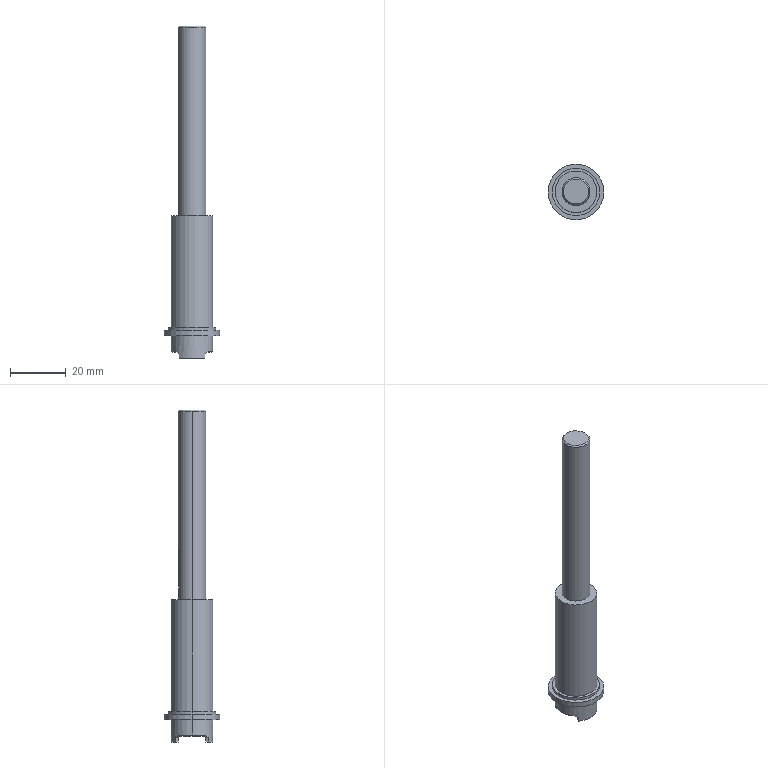Part | STEP file | 11-FG-E03711 | 1 solid | 47 faces | box 20 x 20 x 119 mm | volume 14191 mm3 | plane 19 | cylinder 15 | cone 9 | spline 4 | commonest cylinder face diameters 15 x4 3 x3 3.3 x2 10 x2 17 x2 20 x2
STEP:
#1=CARTESIAN_POINT('',(4.5,0.,119.));
#2=VERTEX_POINT('',#1);
#3=CARTESIAN_POINT('',(-4.5,0.,119.));
#4=VERTEX_POINT('',#3);
#5=CARTESIAN_POINT('',(0.,0.,119.));
#6=DIRECTION('',(0.,0.,1.));
#7=DIRECTION('',(1.,0.,0.));
#8=AXIS2_PLACEMENT_3D('',#5,#6,#7);
#9=CIRCLE('',#8,4.5);
#10=EDGE_CURVE('',#2,#4,#9,.T.);
#11=ORIENTED_EDGE('',*,*,#10,.F.);
#12=CARTESIAN_POINT('',(5.,0.,118.5));
#13=VERTEX_POINT('',#12);
#14=CARTESIAN_POINT('',(4.5,0.,119.));
#15=DIRECTION('',(0.7071,0.,-0.7071));
#16=VECTOR('',#15,1000.);
#17=LINE('',#14,#16);
#18=EDGE_CURVE('',#2,#13,#17,.T.);
#19=ORIENTED_EDGE('',*,*,#18,.T.);
#20=CARTESIAN_POINT('',(-5.,0.,118.5));
#21=VERTEX_POINT('',#20);
#22=CARTESIAN_POINT('',(0.,0.,118.5));
#23=DIRECTION('',(0.,0.,-1.));
#24=DIRECTION('',(1.,0.,0.));
#25=AXIS2_PLACEMENT_3D('',#22,#23,#24);
#26=CIRCLE('',#25,5.);
#27=EDGE_CURVE('',#21,#13,#26,.T.);
#28=ORIENTED_EDGE('',*,*,#27,.F.);
#29=CARTESIAN_POINT('',(-4.5,0.,119.));
#30=DIRECTION('',(-0.7071,0.,-0.7071));
#31=VECTOR('',#30,1000.);
#32=LINE('',#29,#31);
#33=EDGE_CURVE('',#4,#21,#32,.T.);
#34=ORIENTED_EDGE('',*,*,#33,.F.);
#35=EDGE_LOOP('',(#11,#19,#28,#34));
#36=FACE_OUTER_BOUND('',#35,.T.);
#37=CARTESIAN_POINT('',(0.,0.,119.));
#38=DIRECTION('',(0.,0.,-1.));
#39=DIRECTION('',(-1.,0.,0.));
#40=AXIS2_PLACEMENT_3D('',#37,#38,#39);
#41=CONICAL_SURFACE('',#40,4.5,0.7854);
#42=ADVANCED_FACE('',(#36),#41,.T.);
#43=CARTESIAN_POINT('',(1.65,0.,2.5));
#44=VERTEX_POINT('',#43);
#45=CARTESIAN_POINT('',(-1.65,0.,2.5));
#46=VERTEX_POINT('',#45);
#47=CARTESIAN_POINT('',(0.,0.,2.5));
#48=DIRECTION('',(0.,0.,-1.));
#49=DIRECTION('',(-1.,0.,0.));
#50=AXIS2_PLACEMENT_3D('',#47,#48,#49);
#51=CIRCLE('',#50,1.65);
#52=EDGE_CURVE('',#44,#46,#51,.T.);
#53=ORIENTED_EDGE('',*,*,#52,.F.);
#54=CARTESIAN_POINT('',(2.15,0.,2.));
#55=VERTEX_POINT('',#54);
#56=CARTESIAN_POINT('',(1.65,0.,2.5));
#57=DIRECTION('',(0.7071,0.,-0.7071));
#58=VECTOR('',#57,1000.);
#59=LINE('',#56,#58);
#60=EDGE_CURVE('',#44,#55,#59,.T.);
#61=ORIENTED_EDGE('',*,*,#60,.T.);
#62=CARTESIAN_POINT('',(-2.15,0.,2.));
#63=VERTEX_POINT('',#62);
#64=CARTESIAN_POINT('',(0.,0.,2.));
#65=DIRECTION('',(0.,0.,1.));
#66=DIRECTION('',(-1.,0.,0.));
#67=AXIS2_PLACEMENT_3D('',#64,#65,#66);
#68=CIRCLE('',#67,2.15);
#69=EDGE_CURVE('',#63,#55,#68,.T.);
#70=ORIENTED_EDGE('',*,*,#69,.F.);
#71=CARTESIAN_POINT('',(-1.65,0.,2.5));
#72=DIRECTION('',(-0.7071,0.,-0.7071));
#73=VECTOR('',#72,1000.);
#74=LINE('',#71,#73);
#75=EDGE_CURVE('',#46,#63,#74,.T.);
#76=ORIENTED_EDGE('',*,*,#75,.F.);
#77=EDGE_LOOP('',(#53,#61,#70,#76));
#78=FACE_OUTER_BOUND('',#77,.T.);
#79=CARTESIAN_POINT('',(0.,0.,2.5));
#80=DIRECTION('',(0.,0.,-1.));
#81=DIRECTION('',(-1.,0.,0.));
#82=AXIS2_PLACEMENT_3D('',#79,#80,#81);
#83=CONICAL_SURFACE('',#82,1.65,0.7854);
#84=ADVANCED_FACE('',(#78),#83,.F.);
#85=CARTESIAN_POINT('',(7.,0.,2.));
#86=VERTEX_POINT('',#85);
#87=CARTESIAN_POINT('',(5.362,-4.5,2.));
#88=VERTEX_POINT('',#87);
#89=CARTESIAN_POINT('',(0.,0.,2.));
#90=DIRECTION('',(0.,0.,-1.));
#91=DIRECTION('',(-1.,0.,0.));
#92=AXIS2_PLACEMENT_3D('',#89,#90,#91);
#93=CIRCLE('',#92,7.);
#94=EDGE_CURVE('',#86,#88,#93,.T.);
#95=ORIENTED_EDGE('',*,*,#94,.F.);
#96=CARTESIAN_POINT('',(7.5,0.,2.5));
#97=VERTEX_POINT('',#96);
#98=CARTESIAN_POINT('',(7.,0.,2.));
#99=DIRECTION('',(0.7071,0.,0.7071));
#100=VECTOR('',#99,1000.);
#101=LINE('',#98,#100);
#102=EDGE_CURVE('',#86,#97,#101,.T.);
#103=ORIENTED_EDGE('',*,*,#102,.T.);
#104=CARTESIAN_POINT('',(5.745,-4.821,2.5));
#105=VERTEX_POINT('',#104);
#106=CARTESIAN_POINT('',(0.,0.,2.5));
#107=DIRECTION('',(0.,0.,1.));
#108=DIRECTION('',(-1.,0.,0.));
#109=AXIS2_PLACEMENT_3D('',#106,#107,#108);
#110=CIRCLE('',#109,7.5);
#111=EDGE_CURVE('',#105,#97,#110,.T.);
#112=ORIENTED_EDGE('',*,*,#111,.F.);
#113=CARTESIAN_POINT('',(5.362,-4.5,2.));
#114=DIRECTION('',(-0.5416,0.4546,-0.7071));
#115=VECTOR('',#114,1000.);
#116=LINE('',#113,#115);
#117=EDGE_CURVE('',#105,#88,#116,.T.);
#118=ORIENTED_EDGE('',*,*,#117,.T.);
#119=EDGE_LOOP('',(#95,#103,#112,#118));
#120=FACE_OUTER_BOUND('',#119,.T.);
#121=CARTESIAN_POINT('',(0.,0.,2.));
#122=DIRECTION('',(0.,0.,1.));
#123=DIRECTION('',(1.,0.,0.));
#124=AXIS2_PLACEMENT_3D('',#121,#122,#123);
#125=CONICAL_SURFACE('',#124,7.,0.7854);
#126=ADVANCED_FACE('',(#120),#125,.T.);
#127=CARTESIAN_POINT('',(0.,3.,69.5));
#128=VERTEX_POINT('',#127);
#129=CARTESIAN_POINT('',(1.5,3.,68.));
#130=VERTEX_POINT('',#129);
#131=CARTESIAN_POINT('',(0.,3.,68.));
#132=DIRECTION('',(0.,1.,0.));
#133=DIRECTION('',(0.,0.,1.));
#134=AXIS2_PLACEMENT_3D('',#131,#132,#133);
#135=CIRCLE('',#134,1.5);
#136=EDGE_CURVE('',#128,#130,#135,.T.);
#137=ORIENTED_EDGE('',*,*,#136,.F.);
#138=CARTESIAN_POINT('',(0.,5.,69.5));
#139=VERTEX_POINT('',#138);
#140=CARTESIAN_POINT('',(0.,3.,69.5));
#141=DIRECTION('',(0.,1.,0.));
#142=VECTOR('',#141,1000.);
#143=LINE('',#140,#142);
#144=EDGE_CURVE('',#128,#139,#143,.T.);
#145=ORIENTED_EDGE('',*,*,#144,.T.);
#146=CARTESIAN_POINT('',(1.5,4.77,68.));
#147=VERTEX_POINT('',#146);
#148=CARTESIAN_POINT('',(1.5,4.77,68.));
#149=CARTESIAN_POINT('',(1.5,4.77,68.1));
#150=CARTESIAN_POINT('',(1.49,4.773,68.198));
#151=CARTESIAN_POINT('',(1.452,4.785,68.39));
#152=CARTESIAN_POINT('',(1.423,4.794,68.486));
#153=CARTESIAN_POINT('',(1.347,4.815,68.667));
#154=CARTESIAN_POINT('',(1.301,4.828,68.753));
#155=CARTESIAN_POINT('',(1.192,4.856,68.916));
#156=CARTESIAN_POINT('',(1.129,4.871,68.992));
#157=CARTESIAN_POINT('',(0.9226,4.916,69.199));
#158=CARTESIAN_POINT('',(0.7561,4.946,69.31));
#159=CARTESIAN_POINT('',(0.3953,4.988,69.46));
#160=CARTESIAN_POINT('',(0.197,5.,69.5));
#161=CARTESIAN_POINT('',(0.,5.,69.5));
#162=B_SPLINE_CURVE_WITH_KNOTS('',3,(#148,#149,#150,#151,#152,#153,#154,#155,#156,#157,#158,#159,#160,#161),.UNSPECIFIED.,.F.,.F.,(4,2,2,2,2,2,4),(0.,0.0002949,0.0005898,0.0008847,0.00118,0.001769,0.002359),.UNSPECIFIED.);
#163=EDGE_CURVE('',#147,#139,#162,.T.);
#164=ORIENTED_EDGE('',*,*,#163,.F.);
#165=CARTESIAN_POINT('',(1.5,3.,68.));
#166=DIRECTION('',(0.,1.,0.));
#167=VECTOR('',#166,1000.);
#168=LINE('',#165,#167);
#169=EDGE_CURVE('',#130,#147,#168,.T.);
#170=ORIENTED_EDGE('',*,*,#169,.F.);
#171=EDGE_LOOP('',(#137,#145,#164,#170));
#172=FACE_OUTER_BOUND('',#171,.T.);
#173=CARTESIAN_POINT('',(0.,3.,68.));
#174=DIRECTION('',(0.,1.,0.));
#175=DIRECTION('',(0.,0.,1.));
#176=AXIS2_PLACEMENT_3D('',#173,#174,#175);
#177=CYLINDRICAL_SURFACE('',#176,1.5);
#178=ADVANCED_FACE('',(#172),#177,.F.);
#179=CARTESIAN_POINT('',(7.5,0.,51.));
#180=VERTEX_POINT('',#179);
#181=CARTESIAN_POINT('',(-7.5,0.,51.));
#182=VERTEX_POINT('',#181);
#183=CARTESIAN_POINT('',(0.,0.,51.));
#184=DIRECTION('',(0.,0.,1.));
#185=DIRECTION('',(1.,0.,0.));
#186=AXIS2_PLACEMENT_3D('',#183,#184,#185);
#187=CIRCLE('',#186,7.5);
#188=EDGE_CURVE('',#180,#182,#187,.T.);
#189=ORIENTED_EDGE('',*,*,#188,.F.);
#190=CARTESIAN_POINT('',(7.5,0.,11.));
#191=VERTEX_POINT('',#190);
#192=CARTESIAN_POINT('',(7.5,0.,51.));
#193=DIRECTION('',(0.,0.,-1.));
#194=VECTOR('',#193,1000.);
#195=LINE('',#192,#194);
#196=EDGE_CURVE('',#180,#191,#195,.T.);
#197=ORIENTED_EDGE('',*,*,#196,.T.);
#198=CARTESIAN_POINT('',(-7.5,0.,11.));
#199=VERTEX_POINT('',#198);
#200=CARTESIAN_POINT('',(0.,0.,11.));
#201=DIRECTION('',(0.,0.,1.));
#202=DIRECTION('',(1.,0.,0.));
#203=AXIS2_PLACEMENT_3D('',#200,#201,#202);
#204=CIRCLE('',#203,7.5);
#205=EDGE_CURVE('',#191,#199,#204,.T.);
#206=ORIENTED_EDGE('',*,*,#205,.T.);
#207=CARTESIAN_POINT('',(-7.5,0.,51.));
#208=DIRECTION('',(0.,0.,-1.));
#209=VECTOR('',#208,1000.);
#210=LINE('',#207,#209);
#211=EDGE_CURVE('',#182,#199,#210,.T.);
#212=ORIENTED_EDGE('',*,*,#211,.F.);
#213=EDGE_LOOP('',(#189,#197,#206,#212));
#214=FACE_OUTER_BOUND('',#213,.T.);
#215=CARTESIAN_POINT('',(0.,0.,51.));
#216=DIRECTION('',(0.,0.,-1.));
#217=DIRECTION('',(-1.,0.,0.));
#218=AXIS2_PLACEMENT_3D('',#215,#216,#217);
#219=CYLINDRICAL_SURFACE('',#218,7.5);
#220=ADVANCED_FACE('',(#214),#219,.T.);
#221=CARTESIAN_POINT('',(1.5,4.77,53.));
#222=VERTEX_POINT('',#221);
#223=CARTESIAN_POINT('',(1.5,4.77,119.));
#224=DIRECTION('',(0.,0.,1.));
#225=VECTOR('',#224,1000.);
#226=LINE('',#223,#225);
#227=EDGE_CURVE('',#222,#147,#226,.T.);
#228=ORIENTED_EDGE('',*,*,#227,.T.);
#229=ORIENTED_EDGE('',*,*,#163,.T.);
#230=CARTESIAN_POINT('',(-1.5,4.77,68.));
#231=VERTEX_POINT('',#230);
#232=CARTESIAN_POINT('',(0.,5.,69.5));
#233=CARTESIAN_POINT('',(-0.0984,5.,69.5));
#234=CARTESIAN_POINT('',(-0.1984,4.997,69.49));
#235=CARTESIAN_POINT('',(-0.391,4.986,69.451));
#236=CARTESIAN_POINT('',(-0.4848,4.977,69.423));
#237=CARTESIAN_POINT('',(-0.7581,4.946,69.309));
#238=CARTESIAN_POINT('',(-0.9225,4.916,69.199));
#239=CARTESIAN_POINT('',(-1.13,4.871,68.991));
#240=CARTESIAN_POINT('',(-1.192,4.856,68.916));
#241=CARTESIAN_POINT('',(-1.3,4.828,68.754));
#242=CARTESIAN_POINT('',(-1.347,4.815,68.667));
#243=CARTESIAN_POINT('',(-1.46,4.783,68.396));
#244=CARTESIAN_POINT('',(-1.5,4.77,68.199));
#245=CARTESIAN_POINT('',(-1.5,4.77,68.));
#246=B_SPLINE_CURVE_WITH_KNOTS('',3,(#232,#233,#234,#235,#236,#237,#238,#239,#240,#241,#242,#243,#244,#245),.UNSPECIFIED.,.F.,.F.,(4,2,2,2,2,2,4),(0.002359,0.002654,0.002948,0.003537,0.003832,0.004126,0.004715),.UNSPECIFIED.);
#247=EDGE_CURVE('',#139,#231,#246,.T.);
#248=ORIENTED_EDGE('',*,*,#247,.T.);
#249=CARTESIAN_POINT('',(-1.5,4.77,53.));
#250=VERTEX_POINT('',#249);
#251=CARTESIAN_POINT('',(-1.5,4.77,119.));
#252=DIRECTION('',(0.,0.,-1.));
#253=VECTOR('',#252,1000.);
#254=LINE('',#251,#253);
#255=EDGE_CURVE('',#231,#250,#254,.T.);
#256=ORIENTED_EDGE('',*,*,#255,.T.);
#257=CARTESIAN_POINT('',(-1.5,4.77,53.));
#258=CARTESIAN_POINT('',(-1.5,4.77,52.9));
#259=CARTESIAN_POINT('',(-1.49,4.773,52.802));
#260=CARTESIAN_POINT('',(-1.452,4.785,52.61));
#261=CARTESIAN_POINT('',(-1.423,4.794,52.514));
#262=CARTESIAN_POINT('',(-1.347,4.815,52.333));
#263=CARTESIAN_POINT('',(-1.301,4.828,52.247));
#264=CARTESIAN_POINT('',(-1.192,4.856,52.085));
#265=CARTESIAN_POINT('',(-1.129,4.871,52.008));
#266=CARTESIAN_POINT('',(-0.9233,4.916,51.802));
#267=CARTESIAN_POINT('',(-0.7569,4.946,51.69));
#268=CARTESIAN_POINT('',(-0.3965,4.988,51.54));
#269=CARTESIAN_POINT('',(-0.1984,5.,51.5));
#270=CARTESIAN_POINT('',(0.09698,5.,51.5));
#271=CARTESIAN_POINT('',(0.197,4.997,51.51));
#272=CARTESIAN_POINT('',(0.3898,4.986,51.548));
#273=CARTESIAN_POINT('',(0.4837,4.977,51.577));
#274=CARTESIAN_POINT('',(0.7572,4.946,51.69));
#275=CARTESIAN_POINT('',(0.9219,4.916,51.801));
#276=CARTESIAN_POINT('',(1.13,4.871,52.008));
#277=CARTESIAN_POINT('',(1.191,4.856,52.083));
#278=CARTESIAN_POINT('',(1.3,4.828,52.245));
#279=CARTESIAN_POINT('',(1.347,4.815,52.333));
#280=CARTESIAN_POINT('',(1.46,4.783,52.604));
#281=CARTESIAN_POINT('',(1.5,4.77,52.801));
#282=CARTESIAN_POINT('',(1.5,4.77,53.));
#283=B_SPLINE_CURVE_WITH_KNOTS('',3,(#257,#258,#259,#260,#261,#262,#263,#264,#265,#266,#267,#268,#269,#270,#271,#272,#273,#274,#275,#276,#277,#278,#279,#280,#281,#282),.UNSPECIFIED.,.F.,.F.,(4,2,2,2,2,2,2,2,2,2,2,2,4),(0.,0.0002947,0.0005894,0.0008841,0.001179,0.001768,0.002358,0.002652,0.002947,0.003536,0.003831,0.004126,0.004715),.UNSPECIFIED.);
#284=EDGE_CURVE('',#250,#222,#283,.T.);
#285=ORIENTED_EDGE('',*,*,#284,.T.);
#286=EDGE_LOOP('',(#228,#229,#248,#256,#285));
#287=FACE_BOUND('',#286,.T.);
#288=ORIENTED_EDGE('',*,*,#27,.T.);
#289=CARTESIAN_POINT('',(5.,0.,51.));
#290=VERTEX_POINT('',#289);
#291=CARTESIAN_POINT('',(5.,0.,119.));
#292=DIRECTION('',(0.,0.,-1.));
#293=VECTOR('',#292,1000.);
#294=LINE('',#291,#293);
#295=EDGE_CURVE('',#13,#290,#294,.T.);
#296=ORIENTED_EDGE('',*,*,#295,.T.);
#297=CARTESIAN_POINT('',(-5.,0.,51.));
#298=VERTEX_POINT('',#297);
#299=CARTESIAN_POINT('',(0.,0.,51.));
#300=DIRECTION('',(0.,0.,1.));
#301=DIRECTION('',(1.,0.,0.));
#302=AXIS2_PLACEMENT_3D('',#299,#300,#301);
#303=CIRCLE('',#302,5.);
#304=EDGE_CURVE('',#290,#298,#303,.T.);
#305=ORIENTED_EDGE('',*,*,#304,.T.);
#306=CARTESIAN_POINT('',(-5.,0.,119.));
#307=DIRECTION('',(0.,0.,-1.));
#308=VECTOR('',#307,1000.);
#309=LINE('',#306,#308);
#310=EDGE_CURVE('',#21,#298,#309,.T.);
#311=ORIENTED_EDGE('',*,*,#310,.F.);
#312=EDGE_LOOP('',(#288,#296,#305,#311));
#313=FACE_OUTER_BOUND('',#312,.T.);
#314=CARTESIAN_POINT('',(0.,0.,119.));
#315=DIRECTION('',(0.,0.,-1.));
#316=DIRECTION('',(-1.,0.,0.));
#317=AXIS2_PLACEMENT_3D('',#314,#315,#316);
#318=CYLINDRICAL_SURFACE('',#317,5.);
#319=ADVANCED_FACE('',(#287,#313),#318,.T.);
#320=CARTESIAN_POINT('',(8.5,0.,10.));
#321=VERTEX_POINT('',#320);
#322=CARTESIAN_POINT('',(-8.5,0.,10.));
#323=VERTEX_POINT('',#322);
#324=CARTESIAN_POINT('',(0.,0.,10.));
#325=DIRECTION('',(0.,0.,1.));
#326=DIRECTION('',(1.,0.,0.));
#327=AXIS2_PLACEMENT_3D('',#324,#325,#326);
#328=CIRCLE('',#327,8.5);
#329=EDGE_CURVE('',#321,#323,#328,.T.);
#330=ORIENTED_EDGE('',*,*,#329,.T.);
#331=CARTESIAN_POINT('',(-8.5,0.,11.));
#332=VERTEX_POINT('',#331);
#333=CARTESIAN_POINT('',(-8.5,0.,10.));
#334=DIRECTION('',(0.,0.,1.));
#335=VECTOR('',#334,1000.);
#336=LINE('',#333,#335);
#337=EDGE_CURVE('',#323,#332,#336,.T.);
#338=ORIENTED_EDGE('',*,*,#337,.T.);
#339=CARTESIAN_POINT('',(8.5,0.,11.));
#340=VERTEX_POINT('',#339);
#341=CARTESIAN_POINT('',(0.,0.,11.));
#342=DIRECTION('',(0.,0.,1.));
#343=DIRECTION('',(1.,0.,0.));
#344=AXIS2_PLACEMENT_3D('',#341,#342,#343);
#345=CIRCLE('',#344,8.5);
#346=EDGE_CURVE('',#340,#332,#345,.T.);
#347=ORIENTED_EDGE('',*,*,#346,.F.);
#348=CARTESIAN_POINT('',(8.5,0.,10.));
#349=DIRECTION('',(0.,0.,1.));
#350=VECTOR('',#349,1000.);
#351=LINE('',#348,#350);
#352=EDGE_CURVE('',#321,#340,#351,.T.);
#353=ORIENTED_EDGE('',*,*,#352,.F.);
#354=EDGE_LOOP('',(#330,#338,#347,#353));
#355=FACE_OUTER_BOUND('',#354,.T.);
#356=CARTESIAN_POINT('',(0.,0.,10.));
#357=DIRECTION('',(0.,0.,1.));
#358=DIRECTION('',(1.,0.,0.));
#359=AXIS2_PLACEMENT_3D('',#356,#357,#358);
#360=CYLINDRICAL_SURFACE('',#359,8.5);
#361=ADVANCED_FACE('',(#355),#360,.T.);
#362=CARTESIAN_POINT('',(1.65,0.,13.5));
#363=VERTEX_POINT('',#362);
#364=CARTESIAN_POINT('',(-1.65,0.,13.5));
#365=VERTEX_POINT('',#364);
#366=CARTESIAN_POINT('',(0.,0.,13.5));
#367=DIRECTION('',(0.,0.,-1.));
#368=DIRECTION('',(-1.,0.,0.));
#369=AXIS2_PLACEMENT_3D('',#366,#367,#368);
#370=CIRCLE('',#369,1.65);
#371=EDGE_CURVE('',#363,#365,#370,.T.);
#372=ORIENTED_EDGE('',*,*,#371,.F.);
#373=CARTESIAN_POINT('',(1.65,0.,2.));
#374=DIRECTION('',(0.,0.,-1.));
#375=VECTOR('',#374,1000.);
#376=LINE('',#373,#375);
#377=EDGE_CURVE('',#363,#44,#376,.T.);
#378=ORIENTED_EDGE('',*,*,#377,.T.);
#379=ORIENTED_EDGE('',*,*,#52,.T.);
#380=CARTESIAN_POINT('',(-1.65,0.,2.));
#381=DIRECTION('',(0.,0.,-1.));
#382=VECTOR('',#381,1000.);
#383=LINE('',#380,#382);
#384=EDGE_CURVE('',#365,#46,#383,.T.);
#385=ORIENTED_EDGE('',*,*,#384,.F.);
#386=EDGE_LOOP('',(#372,#378,#379,#385));
#387=FACE_OUTER_BOUND('',#386,.T.);
#388=CARTESIAN_POINT('',(0.,0.,2.));
#389=DIRECTION('',(0.,0.,-1.));
#390=DIRECTION('',(-1.,0.,0.));
#391=AXIS2_PLACEMENT_3D('',#388,#389,#390);
#392=CYLINDRICAL_SURFACE('',#391,1.65);
#393=ADVANCED_FACE('',(#387),#392,.F.);
#394=CARTESIAN_POINT('',(0.,0.,14.491));
#395=VERTEX_POINT('',#394);
#396=CARTESIAN_POINT('',(-1.65,0.,13.5));
#397=DIRECTION('',(-0.8572,0.,-0.515));
#398=VECTOR('',#397,1000.);
#399=LINE('',#396,#398);
#400=EDGE_CURVE('',#395,#365,#399,.T.);
#401=ORIENTED_EDGE('',*,*,#400,.F.);
#402=CARTESIAN_POINT('',(1.65,0.,13.5));
#403=DIRECTION('',(0.8572,0.,-0.515));
#404=VECTOR('',#403,1000.);
#405=LINE('',#402,#404);
#406=EDGE_CURVE('',#395,#363,#405,.T.);
#407=ORIENTED_EDGE('',*,*,#406,.T.);
#408=ORIENTED_EDGE('',*,*,#371,.T.);
#409=EDGE_LOOP('',(#401,#407,#408));
#410=FACE_OUTER_BOUND('',#409,.T.);
#411=CARTESIAN_POINT('',(0.,0.,13.5));
#412=DIRECTION('',(0.,0.,-1.));
#413=DIRECTION('',(-1.,0.,0.));
#414=AXIS2_PLACEMENT_3D('',#411,#412,#413);
#415=CONICAL_SURFACE('',#414,1.65,1.03);
#416=ADVANCED_FACE('',(#410),#415,.F.);
#417=CARTESIAN_POINT('',(7.5,0.,8.));
#418=VERTEX_POINT('',#417);
#419=CARTESIAN_POINT('',(-7.5,0.,8.));
#420=VERTEX_POINT('',#419);
#421=CARTESIAN_POINT('',(0.,0.,8.));
#422=DIRECTION('',(0.,0.,1.));
#423=DIRECTION('',(1.,0.,0.));
#424=AXIS2_PLACEMENT_3D('',#421,#422,#423);
#425=CIRCLE('',#424,7.5);
#426=EDGE_CURVE('',#418,#420,#425,.T.);
#427=ORIENTED_EDGE('',*,*,#426,.F.);
#428=CARTESIAN_POINT('',(7.5,0.,8.));
#429=DIRECTION('',(0.,0.,-1.));
#430=VECTOR('',#429,1000.);
#431=LINE('',#428,#430);
#432=EDGE_CURVE('',#418,#97,#431,.T.);
#433=ORIENTED_EDGE('',*,*,#432,.T.);
#434=CARTESIAN_POINT('',(5.745,4.821,2.5));
#435=VERTEX_POINT('',#434);
#436=CARTESIAN_POINT('',(0.,0.,2.5));
#437=DIRECTION('',(0.,0.,1.));
#438=DIRECTION('',(-1.,0.,0.));
#439=AXIS2_PLACEMENT_3D('',#436,#437,#438);
#440=CIRCLE('',#439,7.5);
#441=EDGE_CURVE('',#97,#435,#440,.T.);
#442=ORIENTED_EDGE('',*,*,#441,.T.);
#443=CARTESIAN_POINT('',(4.639,5.893,1.5));
#444=VERTEX_POINT('',#443);
#445=CARTESIAN_POINT('',(4.639,5.893,1.5));
#446=CARTESIAN_POINT('',(4.839,5.736,1.672));
#447=CARTESIAN_POINT('',(5.029,5.57,1.845));
#448=CARTESIAN_POINT('',(5.397,5.215,2.185));
#449=CARTESIAN_POINT('',(5.572,5.027,2.352));
#450=CARTESIAN_POINT('',(5.745,4.821,2.5));
#451=B_SPLINE_CURVE_WITH_KNOTS('',3,(#445,#446,#447,#448,#449,#450),.UNSPECIFIED.,.F.,.F.,(4,2,4),(0.,0.0009195,0.001839),.UNSPECIFIED.);
#452=EDGE_CURVE('',#444,#435,#451,.T.);
#453=ORIENTED_EDGE('',*,*,#452,.F.);
#454=CARTESIAN_POINT('',(4.639,5.893,0.));
#455=VERTEX_POINT('',#454);
#456=CARTESIAN_POINT('',(4.639,5.893,8.));
#457=DIRECTION('',(0.,0.,-1.));
#458=VECTOR('',#457,1000.);
#459=LINE('',#456,#458);
#460=EDGE_CURVE('',#444,#455,#459,.T.);
#461=ORIENTED_EDGE('',*,*,#460,.T.);
#462=CARTESIAN_POINT('',(-4.639,5.893,0.));
#463=VERTEX_POINT('',#462);
#464=CARTESIAN_POINT('',(0.,0.,0.));
#465=DIRECTION('',(0.,0.,1.));
#466=DIRECTION('',(1.,0.,0.));
#467=AXIS2_PLACEMENT_3D('',#464,#465,#466);
#468=CIRCLE('',#467,7.5);
#469=EDGE_CURVE('',#455,#463,#468,.T.);
#470=ORIENTED_EDGE('',*,*,#469,.T.);
#471=CARTESIAN_POINT('',(-4.639,5.893,1.5));
#472=VERTEX_POINT('',#471);
#473=CARTESIAN_POINT('',(-4.639,5.893,8.));
#474=DIRECTION('',(0.,0.,1.));
#475=VECTOR('',#474,1000.);
#476=LINE('',#473,#475);
#477=EDGE_CURVE('',#463,#472,#476,.T.);
#478=ORIENTED_EDGE('',*,*,#477,.T.);
#479=CARTESIAN_POINT('',(-5.745,4.821,2.5));
#480=VERTEX_POINT('',#479);
#481=CARTESIAN_POINT('',(-5.745,4.821,2.5));
#482=CARTESIAN_POINT('',(-5.572,5.027,2.352));
#483=CARTESIAN_POINT('',(-5.396,5.215,2.185));
#484=CARTESIAN_POINT('',(-5.029,5.57,1.845));
#485=CARTESIAN_POINT('',(-4.839,5.736,1.672));
#486=CARTESIAN_POINT('',(-4.639,5.893,1.5));
#487=B_SPLINE_CURVE_WITH_KNOTS('',3,(#481,#482,#483,#484,#485,#486),.UNSPECIFIED.,.F.,.F.,(4,2,4),(0.,0.0009192,0.001838),.UNSPECIFIED.);
#488=EDGE_CURVE('',#480,#472,#487,.T.);
#489=ORIENTED_EDGE('',*,*,#488,.F.);
#490=CARTESIAN_POINT('',(-7.5,0.,2.5));
#491=VERTEX_POINT('',#490);
#492=CARTESIAN_POINT('',(0.,0.,2.5));
#493=DIRECTION('',(0.,0.,1.));
#494=DIRECTION('',(-1.,0.,0.));
#495=AXIS2_PLACEMENT_3D('',#492,#493,#494);
#496=CIRCLE('',#495,7.5);
#497=EDGE_CURVE('',#480,#491,#496,.T.);
#498=ORIENTED_EDGE('',*,*,#497,.T.);
#499=CARTESIAN_POINT('',(-7.5,0.,8.));
#500=DIRECTION('',(0.,0.,-1.));
#501=VECTOR('',#500,1000.);
#502=LINE('',#499,#501);
#503=EDGE_CURVE('',#420,#491,#502,.T.);
#504=ORIENTED_EDGE('',*,*,#503,.F.);
#505=EDGE_LOOP('',(#427,#433,#442,#453,#461,#470,#478,#489,#498,#504));
#506=FACE_OUTER_BOUND('',#505,.T.);
#507=CARTESIAN_POINT('',(0.,0.,8.));
#508=DIRECTION('',(0.,0.,-1.));
#509=DIRECTION('',(-1.,0.,0.));
#510=AXIS2_PLACEMENT_3D('',#507,#508,#509);
#511=CYLINDRICAL_SURFACE('',#510,7.5);
#512=ADVANCED_FACE('',(#506),#511,.T.);
#513=CARTESIAN_POINT('',(10.,0.,10.));
#514=VERTEX_POINT('',#513);
#515=CARTESIAN_POINT('',(-10.,0.,10.));
#516=VERTEX_POINT('',#515);
#517=CARTESIAN_POINT('',(0.,0.,10.));
#518=DIRECTION('',(0.,0.,1.));
#519=DIRECTION('',(1.,0.,0.));
#520=AXIS2_PLACEMENT_3D('',#517,#518,#519);
#521=CIRCLE('',#520,10.);
#522=EDGE_CURVE('',#514,#516,#521,.T.);
#523=ORIENTED_EDGE('',*,*,#522,.F.);
#524=CARTESIAN_POINT('',(10.,0.,8.));
#525=VERTEX_POINT('',#524);
#526=CARTESIAN_POINT('',(10.,0.,11.));
#527=DIRECTION('',(0.,0.,-1.));
#528=VECTOR('',#527,1000.);
#529=LINE('',#526,#528);
#530=EDGE_CURVE('',#514,#525,#529,.T.);
#531=ORIENTED_EDGE('',*,*,#530,.T.);
#532=CARTESIAN_POINT('',(-10.,0.,8.));
#533=VERTEX_POINT('',#532);
#534=CARTESIAN_POINT('',(0.,0.,8.));
#535=DIRECTION('',(0.,0.,1.));
#536=DIRECTION('',(1.,0.,0.));
#537=AXIS2_PLACEMENT_3D('',#534,#535,#536);
#538=CIRCLE('',#537,10.);
#539=EDGE_CURVE('',#525,#533,#538,.T.);
#540=ORIENTED_EDGE('',*,*,#539,.T.);
#541=CARTESIAN_POINT('',(-10.,0.,11.));
#542=DIRECTION('',(0.,0.,-1.));
#543=VECTOR('',#542,1000.);
#544=LINE('',#541,#543);
#545=EDGE_CURVE('',#516,#533,#544,.T.);
#546=ORIENTED_EDGE('',*,*,#545,.F.);
#547=EDGE_LOOP('',(#523,#531,#540,#546));
#548=FACE_OUTER_BOUND('',#547,.T.);
#549=CARTESIAN_POINT('',(0.,0.,11.));
#550=DIRECTION('',(0.,0.,-1.));
#551=DIRECTION('',(-1.,0.,0.));
#552=AXIS2_PLACEMENT_3D('',#549,#550,#551);
#553=CYLINDRICAL_SURFACE('',#552,10.);
#554=ADVANCED_FACE('',(#548),#553,.T.);
#555=ORIENTED_EDGE('',*,*,#530,.F.);
#556=CARTESIAN_POINT('',(0.,0.,10.));
#557=DIRECTION('',(0.,0.,1.));
#558=DIRECTION('',(1.,0.,0.));
#559=AXIS2_PLACEMENT_3D('',#556,#557,#558);
#560=CIRCLE('',#559,10.);
#561=EDGE_CURVE('',#516,#514,#560,.T.);
#562=ORIENTED_EDGE('',*,*,#561,.F.);
#563=ORIENTED_EDGE('',*,*,#545,.T.);
#564=CARTESIAN_POINT('',(0.,0.,8.));
#565=DIRECTION('',(0.,0.,1.));
#566=DIRECTION('',(1.,0.,0.));
#567=AXIS2_PLACEMENT_3D('',#564,#565,#566);
#568=CIRCLE('',#567,10.);
#569=EDGE_CURVE('',#533,#525,#568,.T.);
#570=ORIENTED_EDGE('',*,*,#569,.T.);
#571=EDGE_LOOP('',(#555,#562,#563,#570));
#572=FACE_OUTER_BOUND('',#571,.T.);
#573=CARTESIAN_POINT('',(0.,0.,11.));
#574=DIRECTION('',(0.,0.,-1.));
#575=DIRECTION('',(-1.,0.,0.));
#576=AXIS2_PLACEMENT_3D('',#573,#574,#575);
#577=CYLINDRICAL_SURFACE('',#576,10.);
#578=ADVANCED_FACE('',(#572),#577,.T.);
#579=CARTESIAN_POINT('',(4.33,5.,0.));
#580=VERTEX_POINT('',#579);
#581=CARTESIAN_POINT('',(-4.33,5.,0.));
#582=VERTEX_POINT('',#581);
#583=CARTESIAN_POINT('',(0.,5.,0.));
#584=DIRECTION('',(-1.,0.,0.));
#585=VECTOR('',#584,1000.);
#586=LINE('',#583,#585);
#587=EDGE_CURVE('',#580,#582,#586,.T.);
#588=ORIENTED_EDGE('',*,*,#587,.T.);
#589=CARTESIAN_POINT('',(-4.639,5.893,0.));
#590=DIRECTION('',(-0.3273,0.9449,0.));
#591=VECTOR('',#590,1000.);
#592=LINE('',#589,#591);
#593=EDGE_CURVE('',#582,#463,#592,.T.);
#594=ORIENTED_EDGE('',*,*,#593,.T.);
#595=ORIENTED_EDGE('',*,*,#469,.F.);
#596=CARTESIAN_POINT('',(4.639,5.893,0.));
#597=DIRECTION('',(-0.3273,-0.9449,0.));
#598=VECTOR('',#597,1000.);
#599=LINE('',#596,#598);
#600=EDGE_CURVE('',#455,#580,#599,.T.);
#601=ORIENTED_EDGE('',*,*,#600,.T.);
#602=EDGE_LOOP('',(#588,#594,#595,#601));
#603=FACE_OUTER_BOUND('',#602,.T.);
#604=CARTESIAN_POINT('',(0.,0.,0.));
#605=DIRECTION('',(0.,0.,1.));
#606=DIRECTION('',(1.,0.,0.));
#607=AXIS2_PLACEMENT_3D('',#604,#605,#606);
#608=PLANE('',#607);
#609=ADVANCED_FACE('',(#603),#608,.F.);
#610=ORIENTED_EDGE('',*,*,#432,.F.);
#611=CARTESIAN_POINT('',(0.,0.,8.));
#612=DIRECTION('',(0.,0.,1.));
#613=DIRECTION('',(1.,0.,0.));
#614=AXIS2_PLACEMENT_3D('',#611,#612,#613);
#615=CIRCLE('',#614,7.5);
#616=EDGE_CURVE('',#420,#418,#615,.T.);
#617=ORIENTED_EDGE('',*,*,#616,.F.);
#618=ORIENTED_EDGE('',*,*,#503,.T.);
#619=CARTESIAN_POINT('',(-5.745,-4.821,2.5));
#620=VERTEX_POINT('',#619);
#621=CARTESIAN_POINT('',(0.,0.,2.5));
#622=DIRECTION('',(0.,0.,1.));
#623=DIRECTION('',(-1.,0.,0.));
#624=AXIS2_PLACEMENT_3D('',#621,#622,#623);
#625=CIRCLE('',#624,7.5);
#626=EDGE_CURVE('',#491,#620,#625,.T.);
#627=ORIENTED_EDGE('',*,*,#626,.T.);
#628=CARTESIAN_POINT('',(-4.639,-5.893,1.5));
#629=VERTEX_POINT('',#628);
#630=CARTESIAN_POINT('',(-4.639,-5.893,1.5));
#631=CARTESIAN_POINT('',(-4.839,-5.736,1.672));
#632=CARTESIAN_POINT('',(-5.029,-5.57,1.845));
#633=CARTESIAN_POINT('',(-5.397,-5.215,2.185));
#634=CARTESIAN_POINT('',(-5.572,-5.027,2.352));
#635=CARTESIAN_POINT('',(-5.745,-4.821,2.5));
#636=B_SPLINE_CURVE_WITH_KNOTS('',3,(#630,#631,#632,#633,#634,#635),.UNSPECIFIED.,.F.,.F.,(4,2,4),(0.,0.0009195,0.001839),.UNSPECIFIED.);
#637=EDGE_CURVE('',#629,#620,#636,.T.);
#638=ORIENTED_EDGE('',*,*,#637,.F.);
#639=CARTESIAN_POINT('',(-4.639,-5.893,0.));
#640=VERTEX_POINT('',#639);
#641=CARTESIAN_POINT('',(-4.639,-5.893,8.));
#642=DIRECTION('',(0.,0.,-1.));
#643=VECTOR('',#642,1000.);
#644=LINE('',#641,#643);
#645=EDGE_CURVE('',#629,#640,#644,.T.);
#646=ORIENTED_EDGE('',*,*,#645,.T.);
#647=CARTESIAN_POINT('',(4.639,-5.893,0.));
#648=VERTEX_POINT('',#647);
#649=CARTESIAN_POINT('',(0.,0.,0.));
#650=DIRECTION('',(0.,0.,1.));
#651=DIRECTION('',(1.,0.,0.));
#652=AXIS2_PLACEMENT_3D('',#649,#650,#651);
#653=CIRCLE('',#652,7.5);
#654=EDGE_CURVE('',#640,#648,#653,.T.);
#655=ORIENTED_EDGE('',*,*,#654,.T.);
#656=CARTESIAN_POINT('',(4.639,-5.893,1.5));
#657=VERTEX_POINT('',#656);
#658=CARTESIAN_POINT('',(4.639,-5.893,8.));
#659=DIRECTION('',(0.,0.,1.));
#660=VECTOR('',#659,1000.);
#661=LINE('',#658,#660);
#662=EDGE_CURVE('',#648,#657,#661,.T.);
#663=ORIENTED_EDGE('',*,*,#662,.T.);
#664=CARTESIAN_POINT('',(5.745,-4.821,2.5));
#665=CARTESIAN_POINT('',(5.572,-5.027,2.352));
#666=CARTESIAN_POINT('',(5.396,-5.215,2.185));
#667=CARTESIAN_POINT('',(5.029,-5.57,1.845));
#668=CARTESIAN_POINT('',(4.839,-5.736,1.672));
#669=CARTESIAN_POINT('',(4.639,-5.893,1.5));
#670=B_SPLINE_CURVE_WITH_KNOTS('',3,(#664,#665,#666,#667,#668,#669),.UNSPECIFIED.,.F.,.F.,(4,2,4),(0.,0.0009192,0.001838),.UNSPECIFIED.);
#671=EDGE_CURVE('',#105,#657,#670,.T.);
#672=ORIENTED_EDGE('',*,*,#671,.F.);
#673=ORIENTED_EDGE('',*,*,#111,.T.);
#674=EDGE_LOOP('',(#610,#617,#618,#627,#638,#646,#655,#663,#672,#673));
#675=FACE_OUTER_BOUND('',#674,.T.);
#676=CARTESIAN_POINT('',(0.,0.,8.));
#677=DIRECTION('',(0.,0.,-1.));
#678=DIRECTION('',(-1.,0.,0.));
#679=AXIS2_PLACEMENT_3D('',#676,#677,#678);
#680=CYLINDRICAL_SURFACE('',#679,7.5);
#681=ADVANCED_FACE('',(#675),#680,.T.);
#682=ORIENTED_EDGE('',*,*,#654,.F.);
#683=CARTESIAN_POINT('',(-4.33,-5.,0.));
#684=VERTEX_POINT('',#683);
#685=CARTESIAN_POINT('',(-4.639,-5.893,0.));
#686=DIRECTION('',(0.3273,0.9449,0.));
#687=VECTOR('',#686,1000.);
#688=LINE('',#685,#687);
#689=EDGE_CURVE('',#640,#684,#688,.T.);
#690=ORIENTED_EDGE('',*,*,#689,.T.);
#691=CARTESIAN_POINT('',(4.33,-5.,0.));
#692=VERTEX_POINT('',#691);
#693=CARTESIAN_POINT('',(0.,-5.,0.));
#694=DIRECTION('',(1.,0.,0.));
#695=VECTOR('',#694,1000.);
#696=LINE('',#693,#695);
#697=EDGE_CURVE('',#684,#692,#696,.T.);
#698=ORIENTED_EDGE('',*,*,#697,.T.);
#699=CARTESIAN_POINT('',(4.639,-5.893,0.));
#700=DIRECTION('',(0.3273,-0.9449,0.));
#701=VECTOR('',#700,1000.);
#702=LINE('',#699,#701);
#703=EDGE_CURVE('',#692,#648,#702,.T.);
#704=ORIENTED_EDGE('',*,*,#703,.T.);
#705=EDGE_LOOP('',(#682,#690,#698,#704));
#706=FACE_OUTER_BOUND('',#705,.T.);
#707=CARTESIAN_POINT('',(0.,0.,0.));
#708=DIRECTION('',(0.,0.,1.));
#709=DIRECTION('',(1.,0.,0.));
#710=AXIS2_PLACEMENT_3D('',#707,#708,#709);
#711=PLANE('',#710);
#712=ADVANCED_FACE('',(#706),#711,.F.);
#713=ORIENTED_EDGE('',*,*,#569,.F.);
#714=ORIENTED_EDGE('',*,*,#539,.F.);
#715=EDGE_LOOP('',(#713,#714));
#716=FACE_OUTER_BOUND('',#715,.T.);
#717=ORIENTED_EDGE('',*,*,#616,.T.);
#718=ORIENTED_EDGE('',*,*,#426,.T.);
#719=EDGE_LOOP('',(#717,#718));
#720=FACE_BOUND('',#719,.T.);
#721=CARTESIAN_POINT('',(0.,0.,8.));
#722=DIRECTION('',(0.,0.,1.));
#723=DIRECTION('',(1.,0.,0.));
#724=AXIS2_PLACEMENT_3D('',#721,#722,#723);
#725=PLANE('',#724);
#726=ADVANCED_FACE('',(#716,#720),#725,.F.);
#727=CARTESIAN_POINT('',(-5.362,-4.5,2.));
#728=VERTEX_POINT('',#727);
#729=CARTESIAN_POINT('',(-5.362,4.5,2.));
#730=VERTEX_POINT('',#729);
#731=CARTESIAN_POINT('',(0.,0.,2.));
#732=DIRECTION('',(0.,0.,-1.));
#733=DIRECTION('',(-1.,0.,0.));
#734=AXIS2_PLACEMENT_3D('',#731,#732,#733);
#735=CIRCLE('',#734,7.);
#736=EDGE_CURVE('',#728,#730,#735,.T.);
#737=ORIENTED_EDGE('',*,*,#736,.T.);
#738=CARTESIAN_POINT('',(5.362,4.5,2.));
#739=VERTEX_POINT('',#738);
#740=CARTESIAN_POINT('',(8.66,4.5,2.));
#741=DIRECTION('',(1.,0.,0.));
#742=VECTOR('',#741,1000.);
#743=LINE('',#740,#742);
#744=EDGE_CURVE('',#730,#739,#743,.T.);
#745=ORIENTED_EDGE('',*,*,#744,.T.);
#746=CARTESIAN_POINT('',(0.,0.,2.));
#747=DIRECTION('',(0.,0.,-1.));
#748=DIRECTION('',(-1.,0.,0.));
#749=AXIS2_PLACEMENT_3D('',#746,#747,#748);
#750=CIRCLE('',#749,7.);
#751=EDGE_CURVE('',#739,#86,#750,.T.);
#752=ORIENTED_EDGE('',*,*,#751,.T.);
#753=ORIENTED_EDGE('',*,*,#94,.T.);
#754=CARTESIAN_POINT('',(8.66,-4.5,2.));
#755=DIRECTION('',(-1.,0.,0.));
#756=VECTOR('',#755,1000.);
#757=LINE('',#754,#756);
#758=EDGE_CURVE('',#88,#728,#757,.T.);
#759=ORIENTED_EDGE('',*,*,#758,.T.);
#760=EDGE_LOOP('',(#737,#745,#752,#753,#759));
#761=FACE_OUTER_BOUND('',#760,.T.);
#762=ORIENTED_EDGE('',*,*,#69,.T.);
#763=CARTESIAN_POINT('',(0.,0.,2.));
#764=DIRECTION('',(0.,0.,1.));
#765=DIRECTION('',(-1.,0.,0.));
#766=AXIS2_PLACEMENT_3D('',#763,#764,#765);
#767=CIRCLE('',#766,2.15);
#768=EDGE_CURVE('',#55,#63,#767,.T.);
#769=ORIENTED_EDGE('',*,*,#768,.T.);
#770=EDGE_LOOP('',(#762,#769));
#771=FACE_BOUND('',#770,.T.);
#772=CARTESIAN_POINT('',(8.66,-5.,2.));
#773=DIRECTION('',(0.,0.,-1.));
#774=DIRECTION('',(-1.,0.,0.));
#775=AXIS2_PLACEMENT_3D('',#772,#773,#774);
#776=PLANE('',#775);
#777=ADVANCED_FACE('',(#761,#771),#776,.T.);
#778=CARTESIAN_POINT('',(4.33,5.,1.5));
#779=VERTEX_POINT('',#778);
#780=CARTESIAN_POINT('',(-4.33,5.,1.5));
#781=VERTEX_POINT('',#780);
#782=CARTESIAN_POINT('',(8.66,5.,1.5));
#783=DIRECTION('',(-1.,0.,0.));
#784=VECTOR('',#783,1000.);
#785=LINE('',#782,#784);
#786=EDGE_CURVE('',#779,#781,#785,.T.);
#787=ORIENTED_EDGE('',*,*,#786,.T.);
#788=CARTESIAN_POINT('',(-4.33,5.,2.));
#789=DIRECTION('',(0.,0.,-1.));
#790=VECTOR('',#789,1000.);
#791=LINE('',#788,#790);
#792=EDGE_CURVE('',#781,#582,#791,.T.);
#793=ORIENTED_EDGE('',*,*,#792,.T.);
#794=ORIENTED_EDGE('',*,*,#587,.F.);
#795=CARTESIAN_POINT('',(4.33,5.,2.));
#796=DIRECTION('',(0.,0.,1.));
#797=VECTOR('',#796,1000.);
#798=LINE('',#795,#797);
#799=EDGE_CURVE('',#580,#779,#798,.T.);
#800=ORIENTED_EDGE('',*,*,#799,.T.);
#801=EDGE_LOOP('',(#787,#793,#794,#800));
#802=FACE_OUTER_BOUND('',#801,.T.);
#803=CARTESIAN_POINT('',(8.66,5.,2.));
#804=DIRECTION('',(0.,1.,0.));
#805=DIRECTION('',(0.,0.,1.));
#806=AXIS2_PLACEMENT_3D('',#803,#804,#805);
#807=PLANE('',#806);
#808=ADVANCED_FACE('',(#802),#807,.F.);
#809=ORIENTED_EDGE('',*,*,#697,.F.);
#810=CARTESIAN_POINT('',(-4.33,-5.,1.5));
#811=VERTEX_POINT('',#810);
#812=CARTESIAN_POINT('',(-4.33,-5.,2.));
#813=DIRECTION('',(0.,0.,1.));
#814=VECTOR('',#813,1000.);
#815=LINE('',#812,#814);
#816=EDGE_CURVE('',#684,#811,#815,.T.);
#817=ORIENTED_EDGE('',*,*,#816,.T.);
#818=CARTESIAN_POINT('',(4.33,-5.,1.5));
#819=VERTEX_POINT('',#818);
#820=CARTESIAN_POINT('',(8.66,-5.,1.5));
#821=DIRECTION('',(1.,0.,0.));
#822=VECTOR('',#821,1000.);
#823=LINE('',#820,#822);
#824=EDGE_CURVE('',#811,#819,#823,.T.);
#825=ORIENTED_EDGE('',*,*,#824,.T.);
#826=CARTESIAN_POINT('',(4.33,-5.,2.));
#827=DIRECTION('',(0.,0.,-1.));
#828=VECTOR('',#827,1000.);
#829=LINE('',#826,#828);
#830=EDGE_CURVE('',#819,#692,#829,.T.);
#831=ORIENTED_EDGE('',*,*,#830,.T.);
#832=EDGE_LOOP('',(#809,#817,#825,#831));
#833=FACE_OUTER_BOUND('',#832,.T.);
#834=CARTESIAN_POINT('',(8.66,-5.,2.));
#835=DIRECTION('',(0.,-1.,0.));
#836=DIRECTION('',(0.,0.,-1.));
#837=AXIS2_PLACEMENT_3D('',#834,#835,#836);
#838=PLANE('',#837);
#839=ADVANCED_FACE('',(#833),#838,.F.);
#840=ORIENTED_EDGE('',*,*,#406,.F.);
#841=ORIENTED_EDGE('',*,*,#400,.T.);
#842=CARTESIAN_POINT('',(0.,0.,13.5));
#843=DIRECTION('',(0.,0.,-1.));
#844=DIRECTION('',(-1.,0.,0.));
#845=AXIS2_PLACEMENT_3D('',#842,#843,#844);
#846=CIRCLE('',#845,1.65);
#847=EDGE_CURVE('',#365,#363,#846,.T.);
#848=ORIENTED_EDGE('',*,*,#847,.T.);
#849=EDGE_LOOP('',(#840,#841,#848));
#850=FACE_OUTER_BOUND('',#849,.T.);
#851=CARTESIAN_POINT('',(0.,0.,13.5));
#852=DIRECTION('',(0.,0.,-1.));
#853=DIRECTION('',(-1.,0.,0.));
#854=AXIS2_PLACEMENT_3D('',#851,#852,#853);
#855=CONICAL_SURFACE('',#854,1.65,1.03);
#856=ADVANCED_FACE('',(#850),#855,.F.);
#857=ORIENTED_EDGE('',*,*,#377,.F.);
#858=ORIENTED_EDGE('',*,*,#847,.F.);
#859=ORIENTED_EDGE('',*,*,#384,.T.);
#860=CARTESIAN_POINT('',(0.,0.,2.5));
#861=DIRECTION('',(0.,0.,-1.));
#862=DIRECTION('',(-1.,0.,0.));
#863=AXIS2_PLACEMENT_3D('',#860,#861,#862);
#864=CIRCLE('',#863,1.65);
#865=EDGE_CURVE('',#46,#44,#864,.T.);
#866=ORIENTED_EDGE('',*,*,#865,.T.);
#867=EDGE_LOOP('',(#857,#858,#859,#866));
#868=FACE_OUTER_BOUND('',#867,.T.);
#869=CARTESIAN_POINT('',(0.,0.,2.));
#870=DIRECTION('',(0.,0.,-1.));
#871=DIRECTION('',(-1.,0.,0.));
#872=AXIS2_PLACEMENT_3D('',#869,#870,#871);
#873=CYLINDRICAL_SURFACE('',#872,1.65);
#874=ADVANCED_FACE('',(#868),#873,.F.);
#875=ORIENTED_EDGE('',*,*,#329,.F.);
#876=CARTESIAN_POINT('',(0.,0.,10.));
#877=DIRECTION('',(0.,0.,1.));
#878=DIRECTION('',(1.,0.,0.));
#879=AXIS2_PLACEMENT_3D('',#876,#877,#878);
#880=CIRCLE('',#879,8.5);
#881=EDGE_CURVE('',#323,#321,#880,.T.);
#882=ORIENTED_EDGE('',*,*,#881,.F.);
#883=EDGE_LOOP('',(#875,#882));
#884=FACE_BOUND('',#883,.T.);
#885=ORIENTED_EDGE('',*,*,#561,.T.);
#886=ORIENTED_EDGE('',*,*,#522,.T.);
#887=EDGE_LOOP('',(#885,#886));
#888=FACE_OUTER_BOUND('',#887,.T.);
#889=CARTESIAN_POINT('',(0.,0.,10.));
#890=DIRECTION('',(0.,0.,1.));
#891=DIRECTION('',(1.,0.,0.));
#892=AXIS2_PLACEMENT_3D('',#889,#890,#891);
#893=PLANE('',#892);
#894=ADVANCED_FACE('',(#884,#888),#893,.T.);
#895=ORIENTED_EDGE('',*,*,#337,.F.);
#896=ORIENTED_EDGE('',*,*,#881,.T.);
#897=ORIENTED_EDGE('',*,*,#352,.T.);
#898=CARTESIAN_POINT('',(0.,0.,11.));
#899=DIRECTION('',(0.,0.,1.));
#900=DIRECTION('',(1.,0.,0.));
#901=AXIS2_PLACEMENT_3D('',#898,#899,#900);
#902=CIRCLE('',#901,8.5);
#903=EDGE_CURVE('',#332,#340,#902,.T.);
#904=ORIENTED_EDGE('',*,*,#903,.F.);
#905=EDGE_LOOP('',(#895,#896,#897,#904));
#906=FACE_OUTER_BOUND('',#905,.T.);
#907=CARTESIAN_POINT('',(0.,0.,10.));
#908=DIRECTION('',(0.,0.,1.));
#909=DIRECTION('',(1.,0.,0.));
#910=AXIS2_PLACEMENT_3D('',#907,#908,#909);
#911=CYLINDRICAL_SURFACE('',#910,8.5);
#912=ADVANCED_FACE('',(#906),#911,.T.);
#913=CARTESIAN_POINT('',(0.,0.,119.));
#914=DIRECTION('',(0.,0.,1.));
#915=DIRECTION('',(1.,0.,0.));
#916=AXIS2_PLACEMENT_3D('',#913,#914,#915);
#917=CIRCLE('',#916,4.5);
#918=EDGE_CURVE('',#4,#2,#917,.T.);
#919=ORIENTED_EDGE('',*,*,#918,.T.);
#920=ORIENTED_EDGE('',*,*,#10,.T.);
#921=EDGE_LOOP('',(#919,#920));
#922=FACE_OUTER_BOUND('',#921,.T.);
#923=CARTESIAN_POINT('',(0.,0.,119.));
#924=DIRECTION('',(0.,0.,1.));
#925=DIRECTION('',(1.,0.,0.));
#926=AXIS2_PLACEMENT_3D('',#923,#924,#925);
#927=PLANE('',#926);
#928=ADVANCED_FACE('',(#922),#927,.T.);
#929=ORIENTED_EDGE('',*,*,#295,.F.);
#930=CARTESIAN_POINT('',(0.,0.,118.5));
#931=DIRECTION('',(0.,0.,-1.));
#932=DIRECTION('',(1.,0.,0.));
#933=AXIS2_PLACEMENT_3D('',#930,#931,#932);
#934=CIRCLE('',#933,5.);
#935=EDGE_CURVE('',#13,#21,#934,.T.);
#936=ORIENTED_EDGE('',*,*,#935,.T.);
#937=ORIENTED_EDGE('',*,*,#310,.T.);
#938=CARTESIAN_POINT('',(0.,0.,51.));
#939=DIRECTION('',(0.,0.,1.));
#940=DIRECTION('',(1.,0.,0.));
#941=AXIS2_PLACEMENT_3D('',#938,#939,#940);
#942=CIRCLE('',#941,5.);
#943=EDGE_CURVE('',#298,#290,#942,.T.);
#944=ORIENTED_EDGE('',*,*,#943,.T.);
#945=EDGE_LOOP('',(#929,#936,#937,#944));
#946=FACE_OUTER_BOUND('',#945,.T.);
#947=CARTESIAN_POINT('',(0.,0.,119.));
#948=DIRECTION('',(0.,0.,-1.));
#949=DIRECTION('',(-1.,0.,0.));
#950=AXIS2_PLACEMENT_3D('',#947,#948,#949);
#951=CYLINDRICAL_SURFACE('',#950,5.);
#952=ADVANCED_FACE('',(#946),#951,.T.);
#953=CARTESIAN_POINT('',(0.,0.,51.));
#954=DIRECTION('',(0.,0.,1.));
#955=DIRECTION('',(1.,0.,0.));
#956=AXIS2_PLACEMENT_3D('',#953,#954,#955);
#957=CIRCLE('',#956,7.5);
#958=EDGE_CURVE('',#182,#180,#957,.T.);
#959=ORIENTED_EDGE('',*,*,#958,.T.);
#960=ORIENTED_EDGE('',*,*,#188,.T.);
#961=EDGE_LOOP('',(#959,#960));
#962=FACE_OUTER_BOUND('',#961,.T.);
#963=ORIENTED_EDGE('',*,*,#943,.F.);
#964=ORIENTED_EDGE('',*,*,#304,.F.);
#965=EDGE_LOOP('',(#963,#964));
#966=FACE_BOUND('',#965,.T.);
#967=CARTESIAN_POINT('',(0.,0.,51.));
#968=DIRECTION('',(0.,0.,1.));
#969=DIRECTION('',(1.,0.,0.));
#970=AXIS2_PLACEMENT_3D('',#967,#968,#969);
#971=PLANE('',#970);
#972=ADVANCED_FACE('',(#962,#966),#971,.T.);
#973=ORIENTED_EDGE('',*,*,#196,.F.);
#974=ORIENTED_EDGE('',*,*,#958,.F.);
#975=ORIENTED_EDGE('',*,*,#211,.T.);
#976=CARTESIAN_POINT('',(0.,0.,11.));
#977=DIRECTION('',(0.,0.,1.));
#978=DIRECTION('',(1.,0.,0.));
#979=AXIS2_PLACEMENT_3D('',#976,#977,#978);
#980=CIRCLE('',#979,7.5);
#981=EDGE_CURVE('',#199,#191,#980,.T.);
#982=ORIENTED_EDGE('',*,*,#981,.T.);
#983=EDGE_LOOP('',(#973,#974,#975,#982));
#984=FACE_OUTER_BOUND('',#983,.T.);
#985=CARTESIAN_POINT('',(0.,0.,51.));
#986=DIRECTION('',(0.,0.,-1.));
#987=DIRECTION('',(-1.,0.,0.));
#988=AXIS2_PLACEMENT_3D('',#985,#986,#987);
#989=CYLINDRICAL_SURFACE('',#988,7.5);
#990=ADVANCED_FACE('',(#984),#989,.T.);
#991=ORIENTED_EDGE('',*,*,#981,.F.);
#992=ORIENTED_EDGE('',*,*,#205,.F.);
#993=EDGE_LOOP('',(#991,#992));
#994=FACE_BOUND('',#993,.T.);
#995=ORIENTED_EDGE('',*,*,#346,.T.);
#996=ORIENTED_EDGE('',*,*,#903,.T.);
#997=EDGE_LOOP('',(#995,#996));
#998=FACE_OUTER_BOUND('',#997,.T.);
#999=CARTESIAN_POINT('',(0.,0.,11.));
#1000=DIRECTION('',(0.,0.,1.));
#1001=DIRECTION('',(1.,0.,0.));
#1002=AXIS2_PLACEMENT_3D('',#999,#1000,#1001);
#1003=PLANE('',#1002);
#1004=ADVANCED_FACE('',(#994,#998),#1003,.T.);
#1005=CARTESIAN_POINT('',(-1.5,3.,53.));
#1006=VERTEX_POINT('',#1005);
#1007=CARTESIAN_POINT('',(-1.5,3.,53.));
#1008=DIRECTION('',(0.,1.,0.));
#1009=VECTOR('',#1008,1000.);
#1010=LINE('',#1007,#1009);
#1011=EDGE_CURVE('',#1006,#250,#1010,.T.);
#1012=ORIENTED_EDGE('',*,*,#1011,.F.);
#1013=CARTESIAN_POINT('',(1.5,3.,53.));
#1014=VERTEX_POINT('',#1013);
#1015=CARTESIAN_POINT('',(0.,3.,53.));
#1016=DIRECTION('',(0.,1.,0.));
#1017=DIRECTION('',(0.,0.,1.));
#1018=AXIS2_PLACEMENT_3D('',#1015,#1016,#1017);
#1019=CIRCLE('',#1018,1.5);
#1020=EDGE_CURVE('',#1014,#1006,#1019,.T.);
#1021=ORIENTED_EDGE('',*,*,#1020,.F.);
#1022=CARTESIAN_POINT('',(1.5,3.,53.));
#1023=DIRECTION('',(0.,1.,0.));
#1024=VECTOR('',#1023,1000.);
#1025=LINE('',#1022,#1024);
#1026=EDGE_CURVE('',#1014,#222,#1025,.T.);
#1027=ORIENTED_EDGE('',*,*,#1026,.T.);
#1028=ORIENTED_EDGE('',*,*,#284,.F.);
#1029=EDGE_LOOP('',(#1012,#1021,#1027,#1028));
#1030=FACE_OUTER_BOUND('',#1029,.T.);
#1031=CARTESIAN_POINT('',(0.,3.,53.));
#1032=DIRECTION('',(0.,1.,0.));
#1033=DIRECTION('',(0.,0.,1.));
#1034=AXIS2_PLACEMENT_3D('',#1031,#1032,#1033);
#1035=CYLINDRICAL_SURFACE('',#1034,1.5);
#1036=ADVANCED_FACE('',(#1030),#1035,.F.);
#1037=ORIENTED_EDGE('',*,*,#1026,.F.);
#1038=CARTESIAN_POINT('',(1.5,3.,53.));
#1039=DIRECTION('',(0.,0.,-1.));
#1040=VECTOR('',#1039,1000.);
#1041=LINE('',#1038,#1040);
#1042=EDGE_CURVE('',#130,#1014,#1041,.T.);
#1043=ORIENTED_EDGE('',*,*,#1042,.F.);
#1044=ORIENTED_EDGE('',*,*,#169,.T.);
#1045=ORIENTED_EDGE('',*,*,#227,.F.);
#1046=EDGE_LOOP('',(#1037,#1043,#1044,#1045));
#1047=FACE_OUTER_BOUND('',#1046,.T.);
#1048=CARTESIAN_POINT('',(1.5,3.,53.));
#1049=DIRECTION('',(1.,0.,0.));
#1050=DIRECTION('',(0.,0.,-1.));
#1051=AXIS2_PLACEMENT_3D('',#1048,#1049,#1050);
#1052=PLANE('',#1051);
#1053=ADVANCED_FACE('',(#1047),#1052,.F.);
#1054=ORIENTED_EDGE('',*,*,#144,.F.);
#1055=CARTESIAN_POINT('',(-1.5,3.,68.));
#1056=VERTEX_POINT('',#1055);
#1057=CARTESIAN_POINT('',(0.,3.,68.));
#1058=DIRECTION('',(0.,1.,0.));
#1059=DIRECTION('',(0.,0.,1.));
#1060=AXIS2_PLACEMENT_3D('',#1057,#1058,#1059);
#1061=CIRCLE('',#1060,1.5);
#1062=EDGE_CURVE('',#1056,#128,#1061,.T.);
#1063=ORIENTED_EDGE('',*,*,#1062,.F.);
#1064=CARTESIAN_POINT('',(-1.5,3.,68.));
#1065=DIRECTION('',(0.,1.,0.));
#1066=VECTOR('',#1065,1000.);
#1067=LINE('',#1064,#1066);
#1068=EDGE_CURVE('',#1056,#231,#1067,.T.);
#1069=ORIENTED_EDGE('',*,*,#1068,.T.);
#1070=ORIENTED_EDGE('',*,*,#247,.F.);
#1071=EDGE_LOOP('',(#1054,#1063,#1069,#1070));
#1072=FACE_OUTER_BOUND('',#1071,.T.);
#1073=CARTESIAN_POINT('',(0.,3.,68.));
#1074=DIRECTION('',(0.,1.,0.));
#1075=DIRECTION('',(0.,0.,1.));
#1076=AXIS2_PLACEMENT_3D('',#1073,#1074,#1075);
#1077=CYLINDRICAL_SURFACE('',#1076,1.5);
#1078=ADVANCED_FACE('',(#1072),#1077,.F.);
#1079=ORIENTED_EDGE('',*,*,#1068,.F.);
#1080=CARTESIAN_POINT('',(-1.5,3.,53.));
#1081=DIRECTION('',(0.,0.,1.));
#1082=VECTOR('',#1081,1000.);
#1083=LINE('',#1080,#1082);
#1084=EDGE_CURVE('',#1006,#1056,#1083,.T.);
#1085=ORIENTED_EDGE('',*,*,#1084,.F.);
#1086=ORIENTED_EDGE('',*,*,#1011,.T.);
#1087=ORIENTED_EDGE('',*,*,#255,.F.);
#1088=EDGE_LOOP('',(#1079,#1085,#1086,#1087));
#1089=FACE_OUTER_BOUND('',#1088,.T.);
#1090=CARTESIAN_POINT('',(-1.5,3.,53.));
#1091=DIRECTION('',(-1.,0.,0.));
#1092=DIRECTION('',(0.,0.,1.));
#1093=AXIS2_PLACEMENT_3D('',#1090,#1091,#1092);
#1094=PLANE('',#1093);
#1095=ADVANCED_FACE('',(#1089),#1094,.F.);
#1096=ORIENTED_EDGE('',*,*,#1020,.T.);
#1097=ORIENTED_EDGE('',*,*,#1084,.T.);
#1098=ORIENTED_EDGE('',*,*,#1062,.T.);
#1099=ORIENTED_EDGE('',*,*,#136,.T.);
#1100=ORIENTED_EDGE('',*,*,#1042,.T.);
#1101=EDGE_LOOP('',(#1096,#1097,#1098,#1099,#1100));
#1102=FACE_OUTER_BOUND('',#1101,.T.);
#1103=CARTESIAN_POINT('',(0.,3.,53.));
#1104=DIRECTION('',(0.,1.,0.));
#1105=DIRECTION('',(0.,0.,1.));
#1106=AXIS2_PLACEMENT_3D('',#1103,#1104,#1105);
#1107=PLANE('',#1106);
#1108=ADVANCED_FACE('',(#1102),#1107,.T.);
#1109=CARTESIAN_POINT('',(4.639,-5.893,1.5));
#1110=DIRECTION('',(-0.3273,0.9449,0.));
#1111=VECTOR('',#1110,1000.);
#1112=LINE('',#1109,#1111);
#1113=EDGE_CURVE('',#657,#819,#1112,.T.);
#1114=ORIENTED_EDGE('',*,*,#1113,.F.);
#1115=ORIENTED_EDGE('',*,*,#662,.F.);
#1116=ORIENTED_EDGE('',*,*,#703,.F.);
#1117=ORIENTED_EDGE('',*,*,#830,.F.);
#1118=EDGE_LOOP('',(#1114,#1115,#1116,#1117));
#1119=FACE_OUTER_BOUND('',#1118,.T.);
#1120=CARTESIAN_POINT('',(4.639,-5.893,8.));
#1121=DIRECTION('',(0.9449,0.3273,0.));
#1122=DIRECTION('',(0.,0.,-1.));
#1123=AXIS2_PLACEMENT_3D('',#1120,#1121,#1122);
#1124=PLANE('',#1123);
#1125=ADVANCED_FACE('',(#1119),#1124,.T.);
#1126=ORIENTED_EDGE('',*,*,#671,.T.);
#1127=ORIENTED_EDGE('',*,*,#1113,.T.);
#1128=CARTESIAN_POINT('',(5.362,-4.5,2.));
#1129=CARTESIAN_POINT('',(4.33,-5.,1.5));
#1130=B_SPLINE_CURVE_WITH_KNOTS('',1,(#1128,#1129),.UNSPECIFIED.,.F.,.F.,(2,2),(0.,0.001251),.UNSPECIFIED.);
#1131=EDGE_CURVE('',#88,#819,#1130,.T.);
#1132=ORIENTED_EDGE('',*,*,#1131,.F.);
#1133=ORIENTED_EDGE('',*,*,#117,.F.);
#1134=EDGE_LOOP('',(#1126,#1127,#1132,#1133));
#1135=FACE_OUTER_BOUND('',#1134,.T.);
#1136=CARTESIAN_POINT('',(5.362,-4.5,2.));
#1137=CARTESIAN_POINT('',(4.33,-5.,1.5));
#1138=CARTESIAN_POINT('',(5.745,-4.821,2.5));
#1139=CARTESIAN_POINT('',(4.639,-5.893,1.5));
#1140=CARTESIAN_POINT('',(5.771,-4.843,2.534));
#1141=CARTESIAN_POINT('',(4.66,-5.953,1.5));
#1142=B_SPLINE_SURFACE_WITH_KNOTS('',1,1,((#1136,#1137),(#1138,#1139),(#1140,#1141)),.UNSPECIFIED.,.F.,.F.,.F.,(2,1,2),(2,2),(0.,1.,1.068),(0.,1.),.UNSPECIFIED.);
#1143=ADVANCED_FACE('',(#1135),#1142,.T.);
#1144=ORIENTED_EDGE('',*,*,#689,.F.);
#1145=ORIENTED_EDGE('',*,*,#645,.F.);
#1146=CARTESIAN_POINT('',(-4.33,-5.,1.5));
#1147=DIRECTION('',(-0.3273,-0.9449,0.));
#1148=VECTOR('',#1147,1000.);
#1149=LINE('',#1146,#1148);
#1150=EDGE_CURVE('',#811,#629,#1149,.T.);
#1151=ORIENTED_EDGE('',*,*,#1150,.F.);
#1152=ORIENTED_EDGE('',*,*,#816,.F.);
#1153=EDGE_LOOP('',(#1144,#1145,#1151,#1152));
#1154=FACE_OUTER_BOUND('',#1153,.T.);
#1155=CARTESIAN_POINT('',(-4.639,-5.893,8.));
#1156=DIRECTION('',(0.9449,-0.3273,0.));
#1157=DIRECTION('',(0.,0.,-1.));
#1158=AXIS2_PLACEMENT_3D('',#1155,#1156,#1157);
#1159=PLANE('',#1158);
#1160=ADVANCED_FACE('',(#1154),#1159,.F.);
#1161=ORIENTED_EDGE('',*,*,#1131,.T.);
#1162=ORIENTED_EDGE('',*,*,#824,.F.);
#1163=CARTESIAN_POINT('',(-5.362,-4.5,2.));
#1164=CARTESIAN_POINT('',(-4.33,-5.,1.5));
#1165=B_SPLINE_CURVE_WITH_KNOTS('',1,(#1163,#1164),.UNSPECIFIED.,.F.,.F.,(2,2),(0.,0.001251),.UNSPECIFIED.);
#1166=EDGE_CURVE('',#728,#811,#1165,.T.);
#1167=ORIENTED_EDGE('',*,*,#1166,.F.);
#1168=ORIENTED_EDGE('',*,*,#758,.F.);
#1169=EDGE_LOOP('',(#1161,#1162,#1167,#1168));
#1170=FACE_OUTER_BOUND('',#1169,.T.);
#1171=CARTESIAN_POINT('',(8.66,-4.5,2.));
#1172=DIRECTION('',(0.,-0.7071,0.7071));
#1173=DIRECTION('',(-1.,0.,0.));
#1174=AXIS2_PLACEMENT_3D('',#1171,#1172,#1173);
#1175=PLANE('',#1174);
#1176=ADVANCED_FACE('',(#1170),#1175,.F.);
#1177=ORIENTED_EDGE('',*,*,#102,.F.);
#1178=ORIENTED_EDGE('',*,*,#751,.F.);
#1179=CARTESIAN_POINT('',(5.745,4.821,2.5));
#1180=DIRECTION('',(-0.5416,-0.4546,-0.7071));
#1181=VECTOR('',#1180,1000.);
#1182=LINE('',#1179,#1181);
#1183=EDGE_CURVE('',#435,#739,#1182,.T.);
#1184=ORIENTED_EDGE('',*,*,#1183,.F.);
#1185=ORIENTED_EDGE('',*,*,#441,.F.);
#1186=EDGE_LOOP('',(#1177,#1178,#1184,#1185));
#1187=FACE_OUTER_BOUND('',#1186,.T.);
#1188=CARTESIAN_POINT('',(0.,0.,2.));
#1189=DIRECTION('',(0.,0.,1.));
#1190=DIRECTION('',(1.,0.,0.));
#1191=AXIS2_PLACEMENT_3D('',#1188,#1189,#1190);
#1192=CONICAL_SURFACE('',#1191,7.,0.7854);
#1193=ADVANCED_FACE('',(#1187),#1192,.T.);
#1194=ORIENTED_EDGE('',*,*,#600,.F.);
#1195=ORIENTED_EDGE('',*,*,#460,.F.);
#1196=CARTESIAN_POINT('',(4.33,5.,1.5));
#1197=DIRECTION('',(0.3273,0.9449,0.));
#1198=VECTOR('',#1197,1000.);
#1199=LINE('',#1196,#1198);
#1200=EDGE_CURVE('',#779,#444,#1199,.T.);
#1201=ORIENTED_EDGE('',*,*,#1200,.F.);
#1202=ORIENTED_EDGE('',*,*,#799,.F.);
#1203=EDGE_LOOP('',(#1194,#1195,#1201,#1202));
#1204=FACE_OUTER_BOUND('',#1203,.T.);
#1205=CARTESIAN_POINT('',(4.639,5.893,8.));
#1206=DIRECTION('',(-0.9449,0.3273,0.));
#1207=DIRECTION('',(0.,0.,-1.));
#1208=AXIS2_PLACEMENT_3D('',#1205,#1206,#1207);
#1209=PLANE('',#1208);
#1210=ADVANCED_FACE('',(#1204),#1209,.F.);
#1211=ORIENTED_EDGE('',*,*,#1150,.T.);
#1212=ORIENTED_EDGE('',*,*,#637,.T.);
#1213=CARTESIAN_POINT('',(-5.745,-4.821,2.5));
#1214=DIRECTION('',(-0.5416,-0.4546,0.7071));
#1215=VECTOR('',#1214,1000.);
#1216=LINE('',#1213,#1215);
#1217=EDGE_CURVE('',#728,#620,#1216,.T.);
#1218=ORIENTED_EDGE('',*,*,#1217,.F.);
#1219=ORIENTED_EDGE('',*,*,#1166,.T.);
#1220=EDGE_LOOP('',(#1211,#1212,#1218,#1219));
#1221=FACE_OUTER_BOUND('',#1220,.T.);
#1222=CARTESIAN_POINT('',(-4.33,-5.,1.5));
#1223=CARTESIAN_POINT('',(-5.362,-4.5,2.));
#1224=CARTESIAN_POINT('',(-4.639,-5.893,1.5));
#1225=CARTESIAN_POINT('',(-5.745,-4.821,2.5));
#1226=CARTESIAN_POINT('',(-4.661,-5.955,1.5));
#1227=CARTESIAN_POINT('',(-5.772,-4.844,2.535));
#1228=B_SPLINE_SURFACE_WITH_KNOTS('',1,1,((#1222,#1223),(#1224,#1225),(#1226,#1227)),.UNSPECIFIED.,.F.,.F.,.F.,(2,1,2),(2,2),(0.,1.,1.07),(0.,1.),.UNSPECIFIED.);
#1229=ADVANCED_FACE('',(#1221),#1228,.T.);
#1230=ORIENTED_EDGE('',*,*,#452,.T.);
#1231=ORIENTED_EDGE('',*,*,#1183,.T.);
#1232=CARTESIAN_POINT('',(4.33,5.,1.5));
#1233=CARTESIAN_POINT('',(5.362,4.5,2.));
#1234=B_SPLINE_CURVE_WITH_KNOTS('',1,(#1232,#1233),.UNSPECIFIED.,.F.,.F.,(2,2),(0.,0.001251),.UNSPECIFIED.);
#1235=EDGE_CURVE('',#779,#739,#1234,.T.);
#1236=ORIENTED_EDGE('',*,*,#1235,.F.);
#1237=ORIENTED_EDGE('',*,*,#1200,.T.);
#1238=EDGE_LOOP('',(#1230,#1231,#1236,#1237));
#1239=FACE_OUTER_BOUND('',#1238,.T.);
#1240=CARTESIAN_POINT('',(4.33,5.,1.5));
#1241=CARTESIAN_POINT('',(5.362,4.5,2.));
#1242=CARTESIAN_POINT('',(4.639,5.893,1.5));
#1243=CARTESIAN_POINT('',(5.745,4.821,2.5));
#1244=CARTESIAN_POINT('',(4.661,5.955,1.5));
#1245=CARTESIAN_POINT('',(5.772,4.844,2.535));
#1246=B_SPLINE_SURFACE_WITH_KNOTS('',1,1,((#1240,#1241),(#1242,#1243),(#1244,#1245)),.UNSPECIFIED.,.F.,.F.,.F.,(2,1,2),(2,2),(0.,1.,1.07),(0.,1.),.UNSPECIFIED.);
#1247=ADVANCED_FACE('',(#1239),#1246,.T.);
#1248=ORIENTED_EDGE('',*,*,#1217,.T.);
#1249=ORIENTED_EDGE('',*,*,#626,.F.);
#1250=ORIENTED_EDGE('',*,*,#497,.F.);
#1251=CARTESIAN_POINT('',(-5.362,4.5,2.));
#1252=DIRECTION('',(-0.5416,0.4546,0.7071));
#1253=VECTOR('',#1252,1000.);
#1254=LINE('',#1251,#1253);
#1255=EDGE_CURVE('',#730,#480,#1254,.T.);
#1256=ORIENTED_EDGE('',*,*,#1255,.F.);
#1257=ORIENTED_EDGE('',*,*,#736,.F.);
#1258=EDGE_LOOP('',(#1248,#1249,#1250,#1256,#1257));
#1259=FACE_OUTER_BOUND('',#1258,.T.);
#1260=CARTESIAN_POINT('',(0.,0.,2.));
#1261=DIRECTION('',(0.,0.,1.));
#1262=DIRECTION('',(1.,0.,0.));
#1263=AXIS2_PLACEMENT_3D('',#1260,#1261,#1262);
#1264=CONICAL_SURFACE('',#1263,7.,0.7854);
#1265=ADVANCED_FACE('',(#1259),#1264,.T.);
#1266=ORIENTED_EDGE('',*,*,#1235,.T.);
#1267=ORIENTED_EDGE('',*,*,#744,.F.);
#1268=CARTESIAN_POINT('',(-4.33,5.,1.5));
#1269=CARTESIAN_POINT('',(-5.362,4.5,2.));
#1270=B_SPLINE_CURVE_WITH_KNOTS('',1,(#1268,#1269),.UNSPECIFIED.,.F.,.F.,(2,2),(0.,0.001251),.UNSPECIFIED.);
#1271=EDGE_CURVE('',#781,#730,#1270,.T.);
#1272=ORIENTED_EDGE('',*,*,#1271,.F.);
#1273=ORIENTED_EDGE('',*,*,#786,.F.);
#1274=EDGE_LOOP('',(#1266,#1267,#1272,#1273));
#1275=FACE_OUTER_BOUND('',#1274,.T.);
#1276=CARTESIAN_POINT('',(8.66,4.5,2.));
#1277=DIRECTION('',(0.,0.7071,0.7071));
#1278=DIRECTION('',(1.,0.,0.));
#1279=AXIS2_PLACEMENT_3D('',#1276,#1277,#1278);
#1280=PLANE('',#1279);
#1281=ADVANCED_FACE('',(#1275),#1280,.F.);
#1282=ORIENTED_EDGE('',*,*,#1255,.T.);
#1283=ORIENTED_EDGE('',*,*,#488,.T.);
#1284=CARTESIAN_POINT('',(-4.639,5.893,1.5));
#1285=DIRECTION('',(-0.3273,0.9449,0.));
#1286=VECTOR('',#1285,1000.);
#1287=LINE('',#1284,#1286);
#1288=EDGE_CURVE('',#781,#472,#1287,.T.);
#1289=ORIENTED_EDGE('',*,*,#1288,.F.);
#1290=ORIENTED_EDGE('',*,*,#1271,.T.);
#1291=EDGE_LOOP('',(#1282,#1283,#1289,#1290));
#1292=FACE_OUTER_BOUND('',#1291,.T.);
#1293=CARTESIAN_POINT('',(-5.362,4.5,2.));
#1294=CARTESIAN_POINT('',(-4.33,5.,1.5));
#1295=CARTESIAN_POINT('',(-5.745,4.821,2.5));
#1296=CARTESIAN_POINT('',(-4.639,5.893,1.5));
#1297=CARTESIAN_POINT('',(-5.771,4.843,2.534));
#1298=CARTESIAN_POINT('',(-4.66,5.953,1.5));
#1299=B_SPLINE_SURFACE_WITH_KNOTS('',1,1,((#1293,#1294),(#1295,#1296),(#1297,#1298)),.UNSPECIFIED.,.F.,.F.,.F.,(2,1,2),(2,2),(0.,1.,1.068),(0.,1.),.UNSPECIFIED.);
#1300=ADVANCED_FACE('',(#1292),#1299,.T.);
#1301=ORIENTED_EDGE('',*,*,#593,.F.);
#1302=ORIENTED_EDGE('',*,*,#792,.F.);
#1303=ORIENTED_EDGE('',*,*,#1288,.T.);
#1304=ORIENTED_EDGE('',*,*,#477,.F.);
#1305=EDGE_LOOP('',(#1301,#1302,#1303,#1304));
#1306=FACE_OUTER_BOUND('',#1305,.T.);
#1307=CARTESIAN_POINT('',(-4.639,5.893,8.));
#1308=DIRECTION('',(-0.9449,-0.3273,0.));
#1309=DIRECTION('',(0.,0.,-1.));
#1310=AXIS2_PLACEMENT_3D('',#1307,#1308,#1309);
#1311=PLANE('',#1310);
#1312=ADVANCED_FACE('',(#1306),#1311,.T.);
#1313=ORIENTED_EDGE('',*,*,#60,.F.);
#1314=ORIENTED_EDGE('',*,*,#865,.F.);
#1315=ORIENTED_EDGE('',*,*,#75,.T.);
#1316=ORIENTED_EDGE('',*,*,#768,.F.);
#1317=EDGE_LOOP('',(#1313,#1314,#1315,#1316));
#1318=FACE_OUTER_BOUND('',#1317,.T.);
#1319=CARTESIAN_POINT('',(0.,0.,2.5));
#1320=DIRECTION('',(0.,0.,-1.));
#1321=DIRECTION('',(-1.,0.,0.));
#1322=AXIS2_PLACEMENT_3D('',#1319,#1320,#1321);
#1323=CONICAL_SURFACE('',#1322,1.65,0.7854);
#1324=ADVANCED_FACE('',(#1318),#1323,.F.);
#1325=ORIENTED_EDGE('',*,*,#18,.F.);
#1326=ORIENTED_EDGE('',*,*,#918,.F.);
#1327=ORIENTED_EDGE('',*,*,#33,.T.);
#1328=ORIENTED_EDGE('',*,*,#935,.F.);
#1329=EDGE_LOOP('',(#1325,#1326,#1327,#1328));
#1330=FACE_OUTER_BOUND('',#1329,.T.);
#1331=CARTESIAN_POINT('',(0.,0.,119.));
#1332=DIRECTION('',(0.,0.,-1.));
#1333=DIRECTION('',(-1.,0.,0.));
#1334=AXIS2_PLACEMENT_3D('',#1331,#1332,#1333);
#1335=CONICAL_SURFACE('',#1334,4.5,0.7854);
#1336=ADVANCED_FACE('',(#1330),#1335,.T.);
#1337=CLOSED_SHELL('',(#42,#84,#126,#178,#220,#319,#361,#393,#416,#512,#554,#578,#609,#681,#712,#726,#777,#808,#839,#856,#874,#894,#912,#928,#952,#972,#990,#1004,#1036,#1053,#1078,#1095,#1108,#1125,#1143,#1160,#1176,#1193,#1210,#1229,#1247,#1265,#1281,#1300,#1312,#1324,#1336));
#1338=MANIFOLD_SOLID_BREP('',#1337);
#1339=CARTESIAN_POINT('',(0.,0.,0.));
#1340=DIRECTION('',(0.,0.,1.));
#1341=DIRECTION('',(1.,0.,0.));
#1342=AXIS2_PLACEMENT_3D('',#1339,#1340,#1341);
#1343=(LENGTH_UNIT()NAMED_UNIT(*)SI_UNIT(.MILLI.,.METRE.));
#1344=UNCERTAINTY_MEASURE_WITH_UNIT(LENGTH_MEASURE(0.00001),#1343,'','');
#1345=(NAMED_UNIT(*)PLANE_ANGLE_UNIT()SI_UNIT($,.RADIAN.));
#1346=(NAMED_UNIT(*)SI_UNIT($,.STERADIAN.)SOLID_ANGLE_UNIT());
#1347=(GEOMETRIC_REPRESENTATION_CONTEXT(3)GLOBAL_UNCERTAINTY_ASSIGNED_CONTEXT((#1344))GLOBAL_UNIT_ASSIGNED_CONTEXT((#1343,#1345,#1346))REPRESENTATION_CONTEXT('',''));
#1348=ADVANCED_BREP_SHAPE_REPRESENTATION('',(#1338,#1342),#1347);